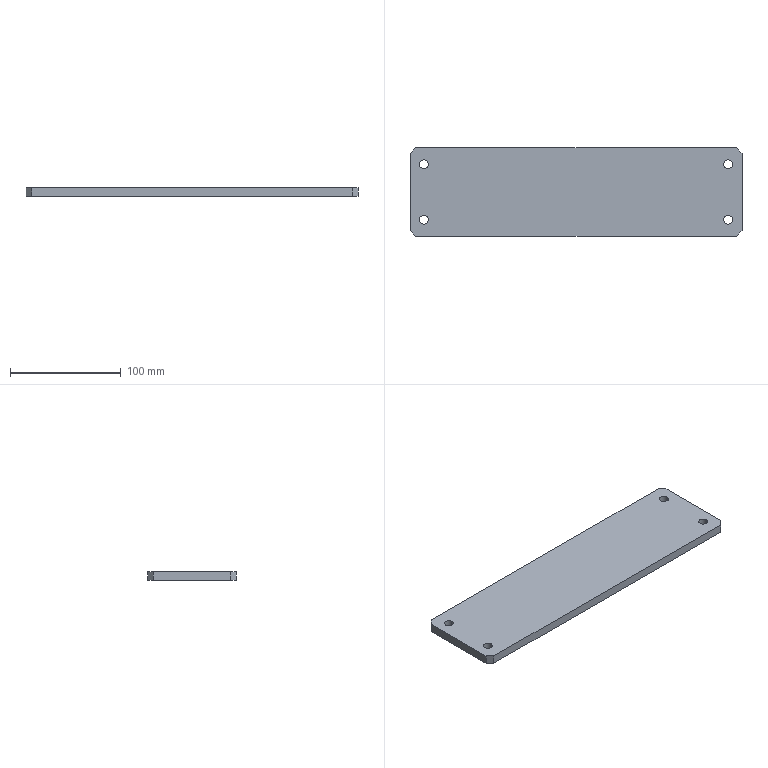Part | SolidWorks | features Chamfer 1, Extrusion 1, ICE 1 | 1 solid | 18 faces | box 300 x 80 x 8 mm | volume 189992 mm3 | plane 10 | cylinder 8 | commonest cylinder face diameters 8 x8
STEP:
#1=CARTESIAN_POINT('',(-141.5,-25.,0.));
#2=VERTEX_POINT('',#1);
#3=CARTESIAN_POINT('',(-133.5,-25.,0.));
#4=VERTEX_POINT('',#3);
#5=CARTESIAN_POINT('',(-137.5,-25.,0.));
#6=DIRECTION('',(0.,0.,1.));
#7=DIRECTION('',(1.,0.,0.));
#8=AXIS2_PLACEMENT_3D('',#5,#6,#7);
#9=CIRCLE('',#8,4.);
#10=EDGE_CURVE('',#2,#4,#9,.T.);
#11=ORIENTED_EDGE('',*,*,#10,.F.);
#12=CARTESIAN_POINT('',(-141.5,-25.,8.));
#13=VERTEX_POINT('',#12);
#14=CARTESIAN_POINT('',(-141.5,-25.,0.));
#15=DIRECTION('',(0.,0.,1.));
#16=VECTOR('',#15,1000.);
#17=LINE('',#14,#16);
#18=EDGE_CURVE('',#2,#13,#17,.T.);
#19=ORIENTED_EDGE('',*,*,#18,.T.);
#20=CARTESIAN_POINT('',(-133.5,-25.,8.));
#21=VERTEX_POINT('',#20);
#22=CARTESIAN_POINT('',(-137.5,-25.,8.));
#23=DIRECTION('',(0.,0.,1.));
#24=DIRECTION('',(1.,0.,0.));
#25=AXIS2_PLACEMENT_3D('',#22,#23,#24);
#26=CIRCLE('',#25,4.);
#27=EDGE_CURVE('',#13,#21,#26,.T.);
#28=ORIENTED_EDGE('',*,*,#27,.T.);
#29=CARTESIAN_POINT('',(-133.5,-25.,0.));
#30=DIRECTION('',(0.,0.,1.));
#31=VECTOR('',#30,1000.);
#32=LINE('',#29,#31);
#33=EDGE_CURVE('',#4,#21,#32,.T.);
#34=ORIENTED_EDGE('',*,*,#33,.F.);
#35=EDGE_LOOP('',(#11,#19,#28,#34));
#36=FACE_OUTER_BOUND('',#35,.T.);
#37=CARTESIAN_POINT('',(-137.5,-25.,0.));
#38=DIRECTION('',(0.,0.,1.));
#39=DIRECTION('',(1.,0.,0.));
#40=AXIS2_PLACEMENT_3D('',#37,#38,#39);
#41=CYLINDRICAL_SURFACE('',#40,4.);
#42=ADVANCED_FACE('',(#36),#41,.F.);
#43=CARTESIAN_POINT('',(133.5,25.,0.));
#44=VERTEX_POINT('',#43);
#45=CARTESIAN_POINT('',(141.5,25.,0.));
#46=VERTEX_POINT('',#45);
#47=CARTESIAN_POINT('',(137.5,25.,0.));
#48=DIRECTION('',(0.,0.,1.));
#49=DIRECTION('',(1.,0.,0.));
#50=AXIS2_PLACEMENT_3D('',#47,#48,#49);
#51=CIRCLE('',#50,4.);
#52=EDGE_CURVE('',#44,#46,#51,.T.);
#53=ORIENTED_EDGE('',*,*,#52,.F.);
#54=CARTESIAN_POINT('',(133.5,25.,8.));
#55=VERTEX_POINT('',#54);
#56=CARTESIAN_POINT('',(133.5,25.,0.));
#57=DIRECTION('',(0.,0.,1.));
#58=VECTOR('',#57,1000.);
#59=LINE('',#56,#58);
#60=EDGE_CURVE('',#44,#55,#59,.T.);
#61=ORIENTED_EDGE('',*,*,#60,.T.);
#62=CARTESIAN_POINT('',(141.5,25.,8.));
#63=VERTEX_POINT('',#62);
#64=CARTESIAN_POINT('',(137.5,25.,8.));
#65=DIRECTION('',(0.,0.,1.));
#66=DIRECTION('',(1.,0.,0.));
#67=AXIS2_PLACEMENT_3D('',#64,#65,#66);
#68=CIRCLE('',#67,4.);
#69=EDGE_CURVE('',#55,#63,#68,.T.);
#70=ORIENTED_EDGE('',*,*,#69,.T.);
#71=CARTESIAN_POINT('',(141.5,25.,0.));
#72=DIRECTION('',(0.,0.,1.));
#73=VECTOR('',#72,1000.);
#74=LINE('',#71,#73);
#75=EDGE_CURVE('',#46,#63,#74,.T.);
#76=ORIENTED_EDGE('',*,*,#75,.F.);
#77=EDGE_LOOP('',(#53,#61,#70,#76));
#78=FACE_OUTER_BOUND('',#77,.T.);
#79=CARTESIAN_POINT('',(137.5,25.,0.));
#80=DIRECTION('',(0.,0.,1.));
#81=DIRECTION('',(1.,0.,0.));
#82=AXIS2_PLACEMENT_3D('',#79,#80,#81);
#83=CYLINDRICAL_SURFACE('',#82,4.);
#84=ADVANCED_FACE('',(#78),#83,.F.);
#85=CARTESIAN_POINT('',(133.5,-25.,0.));
#86=VERTEX_POINT('',#85);
#87=CARTESIAN_POINT('',(141.5,-25.,0.));
#88=VERTEX_POINT('',#87);
#89=CARTESIAN_POINT('',(137.5,-25.,0.));
#90=DIRECTION('',(0.,0.,1.));
#91=DIRECTION('',(1.,0.,0.));
#92=AXIS2_PLACEMENT_3D('',#89,#90,#91);
#93=CIRCLE('',#92,4.);
#94=EDGE_CURVE('',#86,#88,#93,.T.);
#95=ORIENTED_EDGE('',*,*,#94,.F.);
#96=CARTESIAN_POINT('',(133.5,-25.,8.));
#97=VERTEX_POINT('',#96);
#98=CARTESIAN_POINT('',(133.5,-25.,0.));
#99=DIRECTION('',(0.,0.,1.));
#100=VECTOR('',#99,1000.);
#101=LINE('',#98,#100);
#102=EDGE_CURVE('',#86,#97,#101,.T.);
#103=ORIENTED_EDGE('',*,*,#102,.T.);
#104=CARTESIAN_POINT('',(141.5,-25.,8.));
#105=VERTEX_POINT('',#104);
#106=CARTESIAN_POINT('',(137.5,-25.,8.));
#107=DIRECTION('',(0.,0.,1.));
#108=DIRECTION('',(1.,0.,0.));
#109=AXIS2_PLACEMENT_3D('',#106,#107,#108);
#110=CIRCLE('',#109,4.);
#111=EDGE_CURVE('',#97,#105,#110,.T.);
#112=ORIENTED_EDGE('',*,*,#111,.T.);
#113=CARTESIAN_POINT('',(141.5,-25.,0.));
#114=DIRECTION('',(0.,0.,1.));
#115=VECTOR('',#114,1000.);
#116=LINE('',#113,#115);
#117=EDGE_CURVE('',#88,#105,#116,.T.);
#118=ORIENTED_EDGE('',*,*,#117,.F.);
#119=EDGE_LOOP('',(#95,#103,#112,#118));
#120=FACE_OUTER_BOUND('',#119,.T.);
#121=CARTESIAN_POINT('',(137.5,-25.,0.));
#122=DIRECTION('',(0.,0.,1.));
#123=DIRECTION('',(1.,0.,0.));
#124=AXIS2_PLACEMENT_3D('',#121,#122,#123);
#125=CYLINDRICAL_SURFACE('',#124,4.);
#126=ADVANCED_FACE('',(#120),#125,.F.);
#127=CARTESIAN_POINT('',(-141.5,25.,0.));
#128=VERTEX_POINT('',#127);
#129=CARTESIAN_POINT('',(-133.5,25.,0.));
#130=VERTEX_POINT('',#129);
#131=CARTESIAN_POINT('',(-137.5,25.,0.));
#132=DIRECTION('',(0.,0.,1.));
#133=DIRECTION('',(1.,0.,0.));
#134=AXIS2_PLACEMENT_3D('',#131,#132,#133);
#135=CIRCLE('',#134,4.);
#136=EDGE_CURVE('',#128,#130,#135,.T.);
#137=ORIENTED_EDGE('',*,*,#136,.F.);
#138=CARTESIAN_POINT('',(-141.5,25.,8.));
#139=VERTEX_POINT('',#138);
#140=CARTESIAN_POINT('',(-141.5,25.,0.));
#141=DIRECTION('',(0.,0.,1.));
#142=VECTOR('',#141,1000.);
#143=LINE('',#140,#142);
#144=EDGE_CURVE('',#128,#139,#143,.T.);
#145=ORIENTED_EDGE('',*,*,#144,.T.);
#146=CARTESIAN_POINT('',(-133.5,25.,8.));
#147=VERTEX_POINT('',#146);
#148=CARTESIAN_POINT('',(-137.5,25.,8.));
#149=DIRECTION('',(0.,0.,1.));
#150=DIRECTION('',(1.,0.,0.));
#151=AXIS2_PLACEMENT_3D('',#148,#149,#150);
#152=CIRCLE('',#151,4.);
#153=EDGE_CURVE('',#139,#147,#152,.T.);
#154=ORIENTED_EDGE('',*,*,#153,.T.);
#155=CARTESIAN_POINT('',(-133.5,25.,0.));
#156=DIRECTION('',(0.,0.,1.));
#157=VECTOR('',#156,1000.);
#158=LINE('',#155,#157);
#159=EDGE_CURVE('',#130,#147,#158,.T.);
#160=ORIENTED_EDGE('',*,*,#159,.F.);
#161=EDGE_LOOP('',(#137,#145,#154,#160));
#162=FACE_OUTER_BOUND('',#161,.T.);
#163=CARTESIAN_POINT('',(-137.5,25.,0.));
#164=DIRECTION('',(0.,0.,1.));
#165=DIRECTION('',(1.,0.,0.));
#166=AXIS2_PLACEMENT_3D('',#163,#164,#165);
#167=CYLINDRICAL_SURFACE('',#166,4.);
#168=ADVANCED_FACE('',(#162),#167,.F.);
#169=CARTESIAN_POINT('',(-145.,-40.,0.));
#170=VERTEX_POINT('',#169);
#171=CARTESIAN_POINT('',(145.,-40.,0.));
#172=VERTEX_POINT('',#171);
#173=CARTESIAN_POINT('',(-150.,-40.,0.));
#174=DIRECTION('',(1.,0.,0.));
#175=VECTOR('',#174,1000.);
#176=LINE('',#173,#175);
#177=EDGE_CURVE('',#170,#172,#176,.T.);
#178=ORIENTED_EDGE('',*,*,#177,.T.);
#179=CARTESIAN_POINT('',(145.,-40.,8.));
#180=VERTEX_POINT('',#179);
#181=CARTESIAN_POINT('',(145.,-40.,8.));
#182=DIRECTION('',(0.,0.,1.));
#183=VECTOR('',#182,1000.);
#184=LINE('',#181,#183);
#185=EDGE_CURVE('',#172,#180,#184,.T.);
#186=ORIENTED_EDGE('',*,*,#185,.T.);
#187=CARTESIAN_POINT('',(-145.,-40.,8.));
#188=VERTEX_POINT('',#187);
#189=CARTESIAN_POINT('',(-150.,-40.,8.));
#190=DIRECTION('',(1.,0.,0.));
#191=VECTOR('',#190,1000.);
#192=LINE('',#189,#191);
#193=EDGE_CURVE('',#188,#180,#192,.T.);
#194=ORIENTED_EDGE('',*,*,#193,.F.);
#195=CARTESIAN_POINT('',(-145.,-40.,8.));
#196=DIRECTION('',(0.,0.,-1.));
#197=VECTOR('',#196,1000.);
#198=LINE('',#195,#197);
#199=EDGE_CURVE('',#188,#170,#198,.T.);
#200=ORIENTED_EDGE('',*,*,#199,.T.);
#201=EDGE_LOOP('',(#178,#186,#194,#200));
#202=FACE_OUTER_BOUND('',#201,.T.);
#203=CARTESIAN_POINT('',(-150.,-40.,8.));
#204=DIRECTION('',(0.,1.,0.));
#205=DIRECTION('',(0.,0.,1.));
#206=AXIS2_PLACEMENT_3D('',#203,#204,#205);
#207=PLANE('',#206);
#208=ADVANCED_FACE('',(#202),#207,.F.);
#209=CARTESIAN_POINT('',(150.,35.,0.));
#210=VERTEX_POINT('',#209);
#211=CARTESIAN_POINT('',(150.,-35.,0.));
#212=VERTEX_POINT('',#211);
#213=CARTESIAN_POINT('',(150.,40.,0.));
#214=DIRECTION('',(0.,-1.,0.));
#215=VECTOR('',#214,1000.);
#216=LINE('',#213,#215);
#217=EDGE_CURVE('',#210,#212,#216,.T.);
#218=ORIENTED_EDGE('',*,*,#217,.F.);
#219=CARTESIAN_POINT('',(150.,35.,8.));
#220=VERTEX_POINT('',#219);
#221=CARTESIAN_POINT('',(150.,35.,8.));
#222=DIRECTION('',(0.,0.,1.));
#223=VECTOR('',#222,1000.);
#224=LINE('',#221,#223);
#225=EDGE_CURVE('',#210,#220,#224,.T.);
#226=ORIENTED_EDGE('',*,*,#225,.T.);
#227=CARTESIAN_POINT('',(150.,-35.,8.));
#228=VERTEX_POINT('',#227);
#229=CARTESIAN_POINT('',(150.,40.,8.));
#230=DIRECTION('',(0.,-1.,0.));
#231=VECTOR('',#230,1000.);
#232=LINE('',#229,#231);
#233=EDGE_CURVE('',#220,#228,#232,.T.);
#234=ORIENTED_EDGE('',*,*,#233,.T.);
#235=CARTESIAN_POINT('',(150.,-35.,0.));
#236=DIRECTION('',(0.,0.,-1.));
#237=VECTOR('',#236,1000.);
#238=LINE('',#235,#237);
#239=EDGE_CURVE('',#228,#212,#238,.T.);
#240=ORIENTED_EDGE('',*,*,#239,.T.);
#241=EDGE_LOOP('',(#218,#226,#234,#240));
#242=FACE_OUTER_BOUND('',#241,.T.);
#243=CARTESIAN_POINT('',(150.,40.,8.));
#244=DIRECTION('',(1.,0.,0.));
#245=DIRECTION('',(0.,0.,-1.));
#246=AXIS2_PLACEMENT_3D('',#243,#244,#245);
#247=PLANE('',#246);
#248=ADVANCED_FACE('',(#242),#247,.T.);
#249=CARTESIAN_POINT('',(-145.,40.,8.));
#250=VERTEX_POINT('',#249);
#251=CARTESIAN_POINT('',(145.,40.,8.));
#252=VERTEX_POINT('',#251);
#253=CARTESIAN_POINT('',(-150.,40.,8.));
#254=DIRECTION('',(1.,0.,0.));
#255=VECTOR('',#254,1000.);
#256=LINE('',#253,#255);
#257=EDGE_CURVE('',#250,#252,#256,.T.);
#258=ORIENTED_EDGE('',*,*,#257,.T.);
#259=CARTESIAN_POINT('',(145.,40.,0.));
#260=VERTEX_POINT('',#259);
#261=CARTESIAN_POINT('',(145.,40.,8.));
#262=DIRECTION('',(0.,0.,-1.));
#263=VECTOR('',#262,1000.);
#264=LINE('',#261,#263);
#265=EDGE_CURVE('',#252,#260,#264,.T.);
#266=ORIENTED_EDGE('',*,*,#265,.T.);
#267=CARTESIAN_POINT('',(-145.,40.,0.));
#268=VERTEX_POINT('',#267);
#269=CARTESIAN_POINT('',(-150.,40.,0.));
#270=DIRECTION('',(1.,0.,0.));
#271=VECTOR('',#270,1000.);
#272=LINE('',#269,#271);
#273=EDGE_CURVE('',#268,#260,#272,.T.);
#274=ORIENTED_EDGE('',*,*,#273,.F.);
#275=CARTESIAN_POINT('',(-145.,40.,8.));
#276=DIRECTION('',(0.,0.,1.));
#277=VECTOR('',#276,1000.);
#278=LINE('',#275,#277);
#279=EDGE_CURVE('',#268,#250,#278,.T.);
#280=ORIENTED_EDGE('',*,*,#279,.T.);
#281=EDGE_LOOP('',(#258,#266,#274,#280));
#282=FACE_OUTER_BOUND('',#281,.T.);
#283=CARTESIAN_POINT('',(-150.,40.,8.));
#284=DIRECTION('',(0.,1.,0.));
#285=DIRECTION('',(0.,0.,1.));
#286=AXIS2_PLACEMENT_3D('',#283,#284,#285);
#287=PLANE('',#286);
#288=ADVANCED_FACE('',(#282),#287,.T.);
#289=CARTESIAN_POINT('',(-150.,35.,0.));
#290=VERTEX_POINT('',#289);
#291=CARTESIAN_POINT('',(-150.,-35.,0.));
#292=VERTEX_POINT('',#291);
#293=CARTESIAN_POINT('',(-150.,40.,0.));
#294=DIRECTION('',(0.,-1.,0.));
#295=VECTOR('',#294,1000.);
#296=LINE('',#293,#295);
#297=EDGE_CURVE('',#290,#292,#296,.T.);
#298=ORIENTED_EDGE('',*,*,#297,.T.);
#299=CARTESIAN_POINT('',(-150.,-35.,8.));
#300=VERTEX_POINT('',#299);
#301=CARTESIAN_POINT('',(-150.,-35.,8.));
#302=DIRECTION('',(0.,0.,1.));
#303=VECTOR('',#302,1000.);
#304=LINE('',#301,#303);
#305=EDGE_CURVE('',#292,#300,#304,.T.);
#306=ORIENTED_EDGE('',*,*,#305,.T.);
#307=CARTESIAN_POINT('',(-150.,35.,8.));
#308=VERTEX_POINT('',#307);
#309=CARTESIAN_POINT('',(-150.,40.,8.));
#310=DIRECTION('',(0.,-1.,0.));
#311=VECTOR('',#310,1000.);
#312=LINE('',#309,#311);
#313=EDGE_CURVE('',#308,#300,#312,.T.);
#314=ORIENTED_EDGE('',*,*,#313,.F.);
#315=CARTESIAN_POINT('',(-150.,35.,0.));
#316=DIRECTION('',(0.,0.,-1.));
#317=VECTOR('',#316,1000.);
#318=LINE('',#315,#317);
#319=EDGE_CURVE('',#308,#290,#318,.T.);
#320=ORIENTED_EDGE('',*,*,#319,.T.);
#321=EDGE_LOOP('',(#298,#306,#314,#320));
#322=FACE_OUTER_BOUND('',#321,.T.);
#323=CARTESIAN_POINT('',(-150.,40.,8.));
#324=DIRECTION('',(1.,0.,0.));
#325=DIRECTION('',(0.,1.,0.));
#326=AXIS2_PLACEMENT_3D('',#323,#324,#325);
#327=PLANE('',#326);
#328=ADVANCED_FACE('',(#322),#327,.F.);
#329=CARTESIAN_POINT('',(-137.5,-25.,8.));
#330=DIRECTION('',(0.,0.,1.));
#331=DIRECTION('',(1.,0.,0.));
#332=AXIS2_PLACEMENT_3D('',#329,#330,#331);
#333=CIRCLE('',#332,4.);
#334=EDGE_CURVE('',#21,#13,#333,.T.);
#335=ORIENTED_EDGE('',*,*,#334,.F.);
#336=ORIENTED_EDGE('',*,*,#27,.F.);
#337=EDGE_LOOP('',(#335,#336));
#338=FACE_BOUND('',#337,.T.);
#339=CARTESIAN_POINT('',(137.5,25.,8.));
#340=DIRECTION('',(0.,0.,1.));
#341=DIRECTION('',(1.,0.,0.));
#342=AXIS2_PLACEMENT_3D('',#339,#340,#341);
#343=CIRCLE('',#342,4.);
#344=EDGE_CURVE('',#63,#55,#343,.T.);
#345=ORIENTED_EDGE('',*,*,#344,.F.);
#346=ORIENTED_EDGE('',*,*,#69,.F.);
#347=EDGE_LOOP('',(#345,#346));
#348=FACE_BOUND('',#347,.T.);
#349=CARTESIAN_POINT('',(137.5,-25.,8.));
#350=DIRECTION('',(0.,0.,1.));
#351=DIRECTION('',(1.,0.,0.));
#352=AXIS2_PLACEMENT_3D('',#349,#350,#351);
#353=CIRCLE('',#352,4.);
#354=EDGE_CURVE('',#105,#97,#353,.T.);
#355=ORIENTED_EDGE('',*,*,#354,.F.);
#356=ORIENTED_EDGE('',*,*,#111,.F.);
#357=EDGE_LOOP('',(#355,#356));
#358=FACE_BOUND('',#357,.T.);
#359=CARTESIAN_POINT('',(-137.5,25.,8.));
#360=DIRECTION('',(0.,0.,1.));
#361=DIRECTION('',(1.,0.,0.));
#362=AXIS2_PLACEMENT_3D('',#359,#360,#361);
#363=CIRCLE('',#362,4.);
#364=EDGE_CURVE('',#147,#139,#363,.T.);
#365=ORIENTED_EDGE('',*,*,#364,.F.);
#366=ORIENTED_EDGE('',*,*,#153,.F.);
#367=EDGE_LOOP('',(#365,#366));
#368=FACE_BOUND('',#367,.T.);
#369=ORIENTED_EDGE('',*,*,#233,.F.);
#370=CARTESIAN_POINT('',(145.,40.,8.));
#371=DIRECTION('',(-0.7071,0.7071,0.));
#372=VECTOR('',#371,1000.);
#373=LINE('',#370,#372);
#374=EDGE_CURVE('',#220,#252,#373,.T.);
#375=ORIENTED_EDGE('',*,*,#374,.T.);
#376=ORIENTED_EDGE('',*,*,#257,.F.);
#377=CARTESIAN_POINT('',(-150.,35.,8.));
#378=DIRECTION('',(-0.7071,-0.7071,0.));
#379=VECTOR('',#378,1000.);
#380=LINE('',#377,#379);
#381=EDGE_CURVE('',#250,#308,#380,.T.);
#382=ORIENTED_EDGE('',*,*,#381,.T.);
#383=ORIENTED_EDGE('',*,*,#313,.T.);
#384=CARTESIAN_POINT('',(-145.,-40.,8.));
#385=DIRECTION('',(0.7071,-0.7071,0.));
#386=VECTOR('',#385,1000.);
#387=LINE('',#384,#386);
#388=EDGE_CURVE('',#300,#188,#387,.T.);
#389=ORIENTED_EDGE('',*,*,#388,.T.);
#390=ORIENTED_EDGE('',*,*,#193,.T.);
#391=CARTESIAN_POINT('',(150.,-35.,8.));
#392=DIRECTION('',(0.7071,0.7071,0.));
#393=VECTOR('',#392,1000.);
#394=LINE('',#391,#393);
#395=EDGE_CURVE('',#180,#228,#394,.T.);
#396=ORIENTED_EDGE('',*,*,#395,.T.);
#397=EDGE_LOOP('',(#369,#375,#376,#382,#383,#389,#390,#396));
#398=FACE_OUTER_BOUND('',#397,.T.);
#399=CARTESIAN_POINT('',(0.,0.,8.));
#400=DIRECTION('',(0.,0.,-1.));
#401=DIRECTION('',(-1.,0.,0.));
#402=AXIS2_PLACEMENT_3D('',#399,#400,#401);
#403=PLANE('',#402);
#404=ADVANCED_FACE('',(#338,#348,#358,#368,#398),#403,.F.);
#405=CARTESIAN_POINT('',(-137.5,-25.,0.));
#406=DIRECTION('',(0.,0.,1.));
#407=DIRECTION('',(1.,0.,0.));
#408=AXIS2_PLACEMENT_3D('',#405,#406,#407);
#409=CIRCLE('',#408,4.);
#410=EDGE_CURVE('',#4,#2,#409,.T.);
#411=ORIENTED_EDGE('',*,*,#410,.T.);
#412=ORIENTED_EDGE('',*,*,#10,.T.);
#413=EDGE_LOOP('',(#411,#412));
#414=FACE_BOUND('',#413,.T.);
#415=CARTESIAN_POINT('',(137.5,25.,0.));
#416=DIRECTION('',(0.,0.,1.));
#417=DIRECTION('',(1.,0.,0.));
#418=AXIS2_PLACEMENT_3D('',#415,#416,#417);
#419=CIRCLE('',#418,4.);
#420=EDGE_CURVE('',#46,#44,#419,.T.);
#421=ORIENTED_EDGE('',*,*,#420,.T.);
#422=ORIENTED_EDGE('',*,*,#52,.T.);
#423=EDGE_LOOP('',(#421,#422));
#424=FACE_BOUND('',#423,.T.);
#425=CARTESIAN_POINT('',(137.5,-25.,0.));
#426=DIRECTION('',(0.,0.,1.));
#427=DIRECTION('',(1.,0.,0.));
#428=AXIS2_PLACEMENT_3D('',#425,#426,#427);
#429=CIRCLE('',#428,4.);
#430=EDGE_CURVE('',#88,#86,#429,.T.);
#431=ORIENTED_EDGE('',*,*,#430,.T.);
#432=ORIENTED_EDGE('',*,*,#94,.T.);
#433=EDGE_LOOP('',(#431,#432));
#434=FACE_BOUND('',#433,.T.);
#435=CARTESIAN_POINT('',(-137.5,25.,0.));
#436=DIRECTION('',(0.,0.,1.));
#437=DIRECTION('',(1.,0.,0.));
#438=AXIS2_PLACEMENT_3D('',#435,#436,#437);
#439=CIRCLE('',#438,4.);
#440=EDGE_CURVE('',#130,#128,#439,.T.);
#441=ORIENTED_EDGE('',*,*,#440,.T.);
#442=ORIENTED_EDGE('',*,*,#136,.T.);
#443=EDGE_LOOP('',(#441,#442));
#444=FACE_BOUND('',#443,.T.);
#445=ORIENTED_EDGE('',*,*,#273,.T.);
#446=CARTESIAN_POINT('',(92.5,92.5,0.));
#447=DIRECTION('',(0.7071,-0.7071,0.));
#448=VECTOR('',#447,1000.);
#449=LINE('',#446,#448);
#450=EDGE_CURVE('',#260,#210,#449,.T.);
#451=ORIENTED_EDGE('',*,*,#450,.T.);
#452=ORIENTED_EDGE('',*,*,#217,.T.);
#453=CARTESIAN_POINT('',(92.5,-92.5,0.));
#454=DIRECTION('',(-0.7071,-0.7071,0.));
#455=VECTOR('',#454,1000.);
#456=LINE('',#453,#455);
#457=EDGE_CURVE('',#212,#172,#456,.T.);
#458=ORIENTED_EDGE('',*,*,#457,.T.);
#459=ORIENTED_EDGE('',*,*,#177,.F.);
#460=CARTESIAN_POINT('',(-92.5,-92.5,0.));
#461=DIRECTION('',(-0.7071,0.7071,0.));
#462=VECTOR('',#461,1000.);
#463=LINE('',#460,#462);
#464=EDGE_CURVE('',#170,#292,#463,.T.);
#465=ORIENTED_EDGE('',*,*,#464,.T.);
#466=ORIENTED_EDGE('',*,*,#297,.F.);
#467=CARTESIAN_POINT('',(-92.5,92.5,0.));
#468=DIRECTION('',(0.7071,0.7071,0.));
#469=VECTOR('',#468,1000.);
#470=LINE('',#467,#469);
#471=EDGE_CURVE('',#290,#268,#470,.T.);
#472=ORIENTED_EDGE('',*,*,#471,.T.);
#473=EDGE_LOOP('',(#445,#451,#452,#458,#459,#465,#466,#472));
#474=FACE_OUTER_BOUND('',#473,.T.);
#475=CARTESIAN_POINT('',(0.,0.,0.));
#476=DIRECTION('',(0.,0.,-1.));
#477=DIRECTION('',(-1.,0.,0.));
#478=AXIS2_PLACEMENT_3D('',#475,#476,#477);
#479=PLANE('',#478);
#480=ADVANCED_FACE('',(#414,#424,#434,#444,#474),#479,.T.);
#481=ORIENTED_EDGE('',*,*,#144,.F.);
#482=ORIENTED_EDGE('',*,*,#440,.F.);
#483=ORIENTED_EDGE('',*,*,#159,.T.);
#484=ORIENTED_EDGE('',*,*,#364,.T.);
#485=EDGE_LOOP('',(#481,#482,#483,#484));
#486=FACE_OUTER_BOUND('',#485,.T.);
#487=CARTESIAN_POINT('',(-137.5,25.,0.));
#488=DIRECTION('',(0.,0.,1.));
#489=DIRECTION('',(1.,0.,0.));
#490=AXIS2_PLACEMENT_3D('',#487,#488,#489);
#491=CYLINDRICAL_SURFACE('',#490,4.);
#492=ADVANCED_FACE('',(#486),#491,.F.);
#493=ORIENTED_EDGE('',*,*,#102,.F.);
#494=ORIENTED_EDGE('',*,*,#430,.F.);
#495=ORIENTED_EDGE('',*,*,#117,.T.);
#496=ORIENTED_EDGE('',*,*,#354,.T.);
#497=EDGE_LOOP('',(#493,#494,#495,#496));
#498=FACE_OUTER_BOUND('',#497,.T.);
#499=CARTESIAN_POINT('',(137.5,-25.,0.));
#500=DIRECTION('',(0.,0.,1.));
#501=DIRECTION('',(1.,0.,0.));
#502=AXIS2_PLACEMENT_3D('',#499,#500,#501);
#503=CYLINDRICAL_SURFACE('',#502,4.);
#504=ADVANCED_FACE('',(#498),#503,.F.);
#505=ORIENTED_EDGE('',*,*,#60,.F.);
#506=ORIENTED_EDGE('',*,*,#420,.F.);
#507=ORIENTED_EDGE('',*,*,#75,.T.);
#508=ORIENTED_EDGE('',*,*,#344,.T.);
#509=EDGE_LOOP('',(#505,#506,#507,#508));
#510=FACE_OUTER_BOUND('',#509,.T.);
#511=CARTESIAN_POINT('',(137.5,25.,0.));
#512=DIRECTION('',(0.,0.,1.));
#513=DIRECTION('',(1.,0.,0.));
#514=AXIS2_PLACEMENT_3D('',#511,#512,#513);
#515=CYLINDRICAL_SURFACE('',#514,4.);
#516=ADVANCED_FACE('',(#510),#515,.F.);
#517=ORIENTED_EDGE('',*,*,#18,.F.);
#518=ORIENTED_EDGE('',*,*,#410,.F.);
#519=ORIENTED_EDGE('',*,*,#33,.T.);
#520=ORIENTED_EDGE('',*,*,#334,.T.);
#521=EDGE_LOOP('',(#517,#518,#519,#520));
#522=FACE_OUTER_BOUND('',#521,.T.);
#523=CARTESIAN_POINT('',(-137.5,-25.,0.));
#524=DIRECTION('',(0.,0.,1.));
#525=DIRECTION('',(1.,0.,0.));
#526=AXIS2_PLACEMENT_3D('',#523,#524,#525);
#527=CYLINDRICAL_SURFACE('',#526,4.);
#528=ADVANCED_FACE('',(#522),#527,.F.);
#529=ORIENTED_EDGE('',*,*,#374,.F.);
#530=ORIENTED_EDGE('',*,*,#225,.F.);
#531=ORIENTED_EDGE('',*,*,#450,.F.);
#532=ORIENTED_EDGE('',*,*,#265,.F.);
#533=EDGE_LOOP('',(#529,#530,#531,#532));
#534=FACE_OUTER_BOUND('',#533,.T.);
#535=CARTESIAN_POINT('',(145.,40.,8.));
#536=DIRECTION('',(-0.7071,-0.7071,0.));
#537=DIRECTION('',(0.,0.,-1.));
#538=AXIS2_PLACEMENT_3D('',#535,#536,#537);
#539=PLANE('',#538);
#540=ADVANCED_FACE('',(#534),#539,.F.);
#541=ORIENTED_EDGE('',*,*,#395,.F.);
#542=ORIENTED_EDGE('',*,*,#185,.F.);
#543=ORIENTED_EDGE('',*,*,#457,.F.);
#544=ORIENTED_EDGE('',*,*,#239,.F.);
#545=EDGE_LOOP('',(#541,#542,#543,#544));
#546=FACE_OUTER_BOUND('',#545,.T.);
#547=CARTESIAN_POINT('',(150.,-35.,8.));
#548=DIRECTION('',(0.7071,-0.7071,0.));
#549=DIRECTION('',(0.,0.,1.));
#550=AXIS2_PLACEMENT_3D('',#547,#548,#549);
#551=PLANE('',#550);
#552=ADVANCED_FACE('',(#546),#551,.T.);
#553=ORIENTED_EDGE('',*,*,#388,.F.);
#554=ORIENTED_EDGE('',*,*,#305,.F.);
#555=ORIENTED_EDGE('',*,*,#464,.F.);
#556=ORIENTED_EDGE('',*,*,#199,.F.);
#557=EDGE_LOOP('',(#553,#554,#555,#556));
#558=FACE_OUTER_BOUND('',#557,.T.);
#559=CARTESIAN_POINT('',(-145.,-40.,8.));
#560=DIRECTION('',(0.7071,0.7071,0.));
#561=DIRECTION('',(0.,0.,-1.));
#562=AXIS2_PLACEMENT_3D('',#559,#560,#561);
#563=PLANE('',#562);
#564=ADVANCED_FACE('',(#558),#563,.F.);
#565=ORIENTED_EDGE('',*,*,#381,.F.);
#566=ORIENTED_EDGE('',*,*,#279,.F.);
#567=ORIENTED_EDGE('',*,*,#471,.F.);
#568=ORIENTED_EDGE('',*,*,#319,.F.);
#569=EDGE_LOOP('',(#565,#566,#567,#568));
#570=FACE_OUTER_BOUND('',#569,.T.);
#571=CARTESIAN_POINT('',(-150.,35.,8.));
#572=DIRECTION('',(-0.7071,0.7071,0.));
#573=DIRECTION('',(0.,0.,1.));
#574=AXIS2_PLACEMENT_3D('',#571,#572,#573);
#575=PLANE('',#574);
#576=ADVANCED_FACE('',(#570),#575,.T.);
#577=CLOSED_SHELL('',(#42,#84,#126,#168,#208,#248,#288,#328,#404,#480,#492,#504,#516,#528,#540,#552,#564,#576));
#578=MANIFOLD_SOLID_BREP('',#577);
#579=CARTESIAN_POINT('',(0.,0.,0.));
#580=DIRECTION('',(0.,0.,1.));
#581=DIRECTION('',(1.,0.,0.));
#582=AXIS2_PLACEMENT_3D('',#579,#580,#581);
#583=(LENGTH_UNIT()NAMED_UNIT(*)SI_UNIT(.MILLI.,.METRE.));
#584=UNCERTAINTY_MEASURE_WITH_UNIT(LENGTH_MEASURE(0.00001),#583,'','');
#585=(NAMED_UNIT(*)PLANE_ANGLE_UNIT()SI_UNIT($,.RADIAN.));
#586=(NAMED_UNIT(*)SI_UNIT($,.STERADIAN.)SOLID_ANGLE_UNIT());
#587=(GEOMETRIC_REPRESENTATION_CONTEXT(3)GLOBAL_UNCERTAINTY_ASSIGNED_CONTEXT((#584))GLOBAL_UNIT_ASSIGNED_CONTEXT((#583,#585,#586))REPRESENTATION_CONTEXT('',''));
#588=ADVANCED_BREP_SHAPE_REPRESENTATION('',(#578,#582),#587);